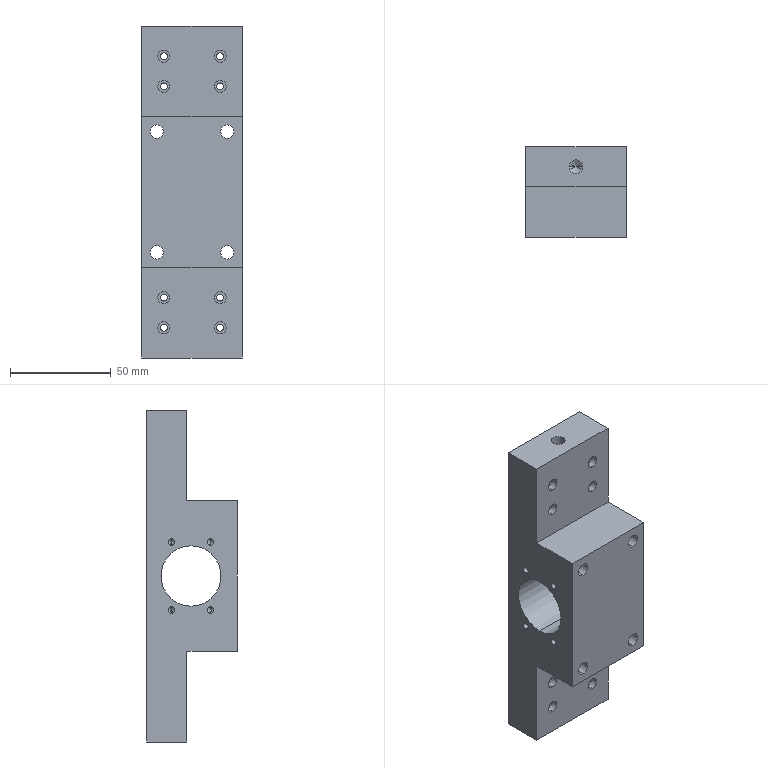Part | STEP file | X77-04007 | 1 solid | 92 faces | box 50 x 45 x 165 mm | volume 212521 mm3 | cylinder 60 | plane 22 | cone 10 | commonest cylinder face diameters 3.4 x16 6 x16 3.3 x8 6.6 x8 11 x8 6.8 x2